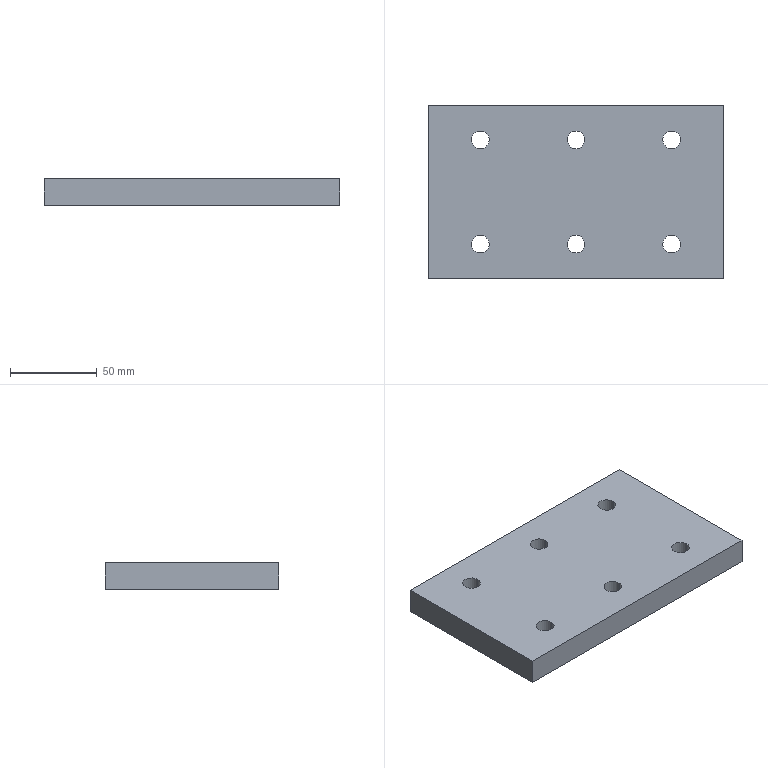Part | SolidWorks | features Extrusion 1, HoleWzd 1 | 1 solid | 18 faces | box 170 x 100 x 15 mm | volume 247646 mm3 | cylinder 12 | plane 6 | commonest cylinder face diameters 10.2 x12
STEP:
#1=CARTESIAN_POINT('',(-60.1,30.,0.));
#2=VERTEX_POINT('',#1);
#3=CARTESIAN_POINT('',(-49.9,30.,0.));
#4=VERTEX_POINT('',#3);
#5=CARTESIAN_POINT('',(-55.,30.,0.));
#6=DIRECTION('',(0.,0.,1.));
#7=DIRECTION('',(1.,0.,0.));
#8=AXIS2_PLACEMENT_3D('',#5,#6,#7);
#9=CIRCLE('',#8,5.1);
#10=EDGE_CURVE('',#2,#4,#9,.T.);
#11=ORIENTED_EDGE('',*,*,#10,.F.);
#12=CARTESIAN_POINT('',(-60.1,30.,15.));
#13=VERTEX_POINT('',#12);
#14=CARTESIAN_POINT('',(-60.1,30.,15.));
#15=DIRECTION('',(0.,0.,1.));
#16=VECTOR('',#15,1000.);
#17=LINE('',#14,#16);
#18=EDGE_CURVE('',#2,#13,#17,.T.);
#19=ORIENTED_EDGE('',*,*,#18,.T.);
#20=CARTESIAN_POINT('',(-49.9,30.,15.));
#21=VERTEX_POINT('',#20);
#22=CARTESIAN_POINT('',(-55.,30.,15.));
#23=DIRECTION('',(0.,0.,1.));
#24=DIRECTION('',(1.,0.,0.));
#25=AXIS2_PLACEMENT_3D('',#22,#23,#24);
#26=CIRCLE('',#25,5.1);
#27=EDGE_CURVE('',#13,#21,#26,.T.);
#28=ORIENTED_EDGE('',*,*,#27,.T.);
#29=CARTESIAN_POINT('',(-49.9,30.,15.));
#30=DIRECTION('',(0.,0.,1.));
#31=VECTOR('',#30,1000.);
#32=LINE('',#29,#31);
#33=EDGE_CURVE('',#4,#21,#32,.T.);
#34=ORIENTED_EDGE('',*,*,#33,.F.);
#35=EDGE_LOOP('',(#11,#19,#28,#34));
#36=FACE_OUTER_BOUND('',#35,.T.);
#37=CARTESIAN_POINT('',(-55.,30.,15.));
#38=DIRECTION('',(0.,0.,1.));
#39=DIRECTION('',(1.,0.,0.));
#40=AXIS2_PLACEMENT_3D('',#37,#38,#39);
#41=CYLINDRICAL_SURFACE('',#40,5.1);
#42=ADVANCED_FACE('',(#36),#41,.F.);
#43=CARTESIAN_POINT('',(-5.1,30.,0.));
#44=VERTEX_POINT('',#43);
#45=CARTESIAN_POINT('',(5.1,30.,0.));
#46=VERTEX_POINT('',#45);
#47=CARTESIAN_POINT('',(0.,30.,0.));
#48=DIRECTION('',(0.,0.,1.));
#49=DIRECTION('',(1.,0.,0.));
#50=AXIS2_PLACEMENT_3D('',#47,#48,#49);
#51=CIRCLE('',#50,5.1);
#52=EDGE_CURVE('',#44,#46,#51,.T.);
#53=ORIENTED_EDGE('',*,*,#52,.F.);
#54=CARTESIAN_POINT('',(-5.1,30.,15.));
#55=VERTEX_POINT('',#54);
#56=CARTESIAN_POINT('',(-5.1,30.,15.));
#57=DIRECTION('',(0.,0.,1.));
#58=VECTOR('',#57,1000.);
#59=LINE('',#56,#58);
#60=EDGE_CURVE('',#44,#55,#59,.T.);
#61=ORIENTED_EDGE('',*,*,#60,.T.);
#62=CARTESIAN_POINT('',(5.1,30.,15.));
#63=VERTEX_POINT('',#62);
#64=CARTESIAN_POINT('',(0.,30.,15.));
#65=DIRECTION('',(0.,0.,1.));
#66=DIRECTION('',(1.,0.,0.));
#67=AXIS2_PLACEMENT_3D('',#64,#65,#66);
#68=CIRCLE('',#67,5.1);
#69=EDGE_CURVE('',#55,#63,#68,.T.);
#70=ORIENTED_EDGE('',*,*,#69,.T.);
#71=CARTESIAN_POINT('',(5.1,30.,15.));
#72=DIRECTION('',(0.,0.,1.));
#73=VECTOR('',#72,1000.);
#74=LINE('',#71,#73);
#75=EDGE_CURVE('',#46,#63,#74,.T.);
#76=ORIENTED_EDGE('',*,*,#75,.F.);
#77=EDGE_LOOP('',(#53,#61,#70,#76));
#78=FACE_OUTER_BOUND('',#77,.T.);
#79=CARTESIAN_POINT('',(0.,30.,15.));
#80=DIRECTION('',(0.,0.,1.));
#81=DIRECTION('',(1.,0.,0.));
#82=AXIS2_PLACEMENT_3D('',#79,#80,#81);
#83=CYLINDRICAL_SURFACE('',#82,5.1);
#84=ADVANCED_FACE('',(#78),#83,.F.);
#85=CARTESIAN_POINT('',(49.9,30.,0.));
#86=VERTEX_POINT('',#85);
#87=CARTESIAN_POINT('',(60.1,30.,0.));
#88=VERTEX_POINT('',#87);
#89=CARTESIAN_POINT('',(55.,30.,0.));
#90=DIRECTION('',(0.,0.,1.));
#91=DIRECTION('',(1.,0.,0.));
#92=AXIS2_PLACEMENT_3D('',#89,#90,#91);
#93=CIRCLE('',#92,5.1);
#94=EDGE_CURVE('',#86,#88,#93,.T.);
#95=ORIENTED_EDGE('',*,*,#94,.F.);
#96=CARTESIAN_POINT('',(49.9,30.,15.));
#97=VERTEX_POINT('',#96);
#98=CARTESIAN_POINT('',(49.9,30.,15.));
#99=DIRECTION('',(0.,0.,1.));
#100=VECTOR('',#99,1000.);
#101=LINE('',#98,#100);
#102=EDGE_CURVE('',#86,#97,#101,.T.);
#103=ORIENTED_EDGE('',*,*,#102,.T.);
#104=CARTESIAN_POINT('',(60.1,30.,15.));
#105=VERTEX_POINT('',#104);
#106=CARTESIAN_POINT('',(55.,30.,15.));
#107=DIRECTION('',(0.,0.,1.));
#108=DIRECTION('',(1.,0.,0.));
#109=AXIS2_PLACEMENT_3D('',#106,#107,#108);
#110=CIRCLE('',#109,5.1);
#111=EDGE_CURVE('',#97,#105,#110,.T.);
#112=ORIENTED_EDGE('',*,*,#111,.T.);
#113=CARTESIAN_POINT('',(60.1,30.,15.));
#114=DIRECTION('',(0.,0.,1.));
#115=VECTOR('',#114,1000.);
#116=LINE('',#113,#115);
#117=EDGE_CURVE('',#88,#105,#116,.T.);
#118=ORIENTED_EDGE('',*,*,#117,.F.);
#119=EDGE_LOOP('',(#95,#103,#112,#118));
#120=FACE_OUTER_BOUND('',#119,.T.);
#121=CARTESIAN_POINT('',(55.,30.,15.));
#122=DIRECTION('',(0.,0.,1.));
#123=DIRECTION('',(1.,0.,0.));
#124=AXIS2_PLACEMENT_3D('',#121,#122,#123);
#125=CYLINDRICAL_SURFACE('',#124,5.1);
#126=ADVANCED_FACE('',(#120),#125,.F.);
#127=CARTESIAN_POINT('',(49.9,-30.,0.));
#128=VERTEX_POINT('',#127);
#129=CARTESIAN_POINT('',(60.1,-30.,0.));
#130=VERTEX_POINT('',#129);
#131=CARTESIAN_POINT('',(55.,-30.,0.));
#132=DIRECTION('',(0.,0.,1.));
#133=DIRECTION('',(1.,0.,0.));
#134=AXIS2_PLACEMENT_3D('',#131,#132,#133);
#135=CIRCLE('',#134,5.1);
#136=EDGE_CURVE('',#128,#130,#135,.T.);
#137=ORIENTED_EDGE('',*,*,#136,.F.);
#138=CARTESIAN_POINT('',(49.9,-30.,15.));
#139=VERTEX_POINT('',#138);
#140=CARTESIAN_POINT('',(49.9,-30.,15.));
#141=DIRECTION('',(0.,0.,1.));
#142=VECTOR('',#141,1000.);
#143=LINE('',#140,#142);
#144=EDGE_CURVE('',#128,#139,#143,.T.);
#145=ORIENTED_EDGE('',*,*,#144,.T.);
#146=CARTESIAN_POINT('',(60.1,-30.,15.));
#147=VERTEX_POINT('',#146);
#148=CARTESIAN_POINT('',(55.,-30.,15.));
#149=DIRECTION('',(0.,0.,1.));
#150=DIRECTION('',(1.,0.,0.));
#151=AXIS2_PLACEMENT_3D('',#148,#149,#150);
#152=CIRCLE('',#151,5.1);
#153=EDGE_CURVE('',#139,#147,#152,.T.);
#154=ORIENTED_EDGE('',*,*,#153,.T.);
#155=CARTESIAN_POINT('',(60.1,-30.,15.));
#156=DIRECTION('',(0.,0.,1.));
#157=VECTOR('',#156,1000.);
#158=LINE('',#155,#157);
#159=EDGE_CURVE('',#130,#147,#158,.T.);
#160=ORIENTED_EDGE('',*,*,#159,.F.);
#161=EDGE_LOOP('',(#137,#145,#154,#160));
#162=FACE_OUTER_BOUND('',#161,.T.);
#163=CARTESIAN_POINT('',(55.,-30.,15.));
#164=DIRECTION('',(0.,0.,1.));
#165=DIRECTION('',(1.,0.,0.));
#166=AXIS2_PLACEMENT_3D('',#163,#164,#165);
#167=CYLINDRICAL_SURFACE('',#166,5.1);
#168=ADVANCED_FACE('',(#162),#167,.F.);
#169=CARTESIAN_POINT('',(-5.1,-30.,0.));
#170=VERTEX_POINT('',#169);
#171=CARTESIAN_POINT('',(5.1,-30.,0.));
#172=VERTEX_POINT('',#171);
#173=CARTESIAN_POINT('',(0.,-30.,0.));
#174=DIRECTION('',(0.,0.,1.));
#175=DIRECTION('',(1.,0.,0.));
#176=AXIS2_PLACEMENT_3D('',#173,#174,#175);
#177=CIRCLE('',#176,5.1);
#178=EDGE_CURVE('',#170,#172,#177,.T.);
#179=ORIENTED_EDGE('',*,*,#178,.F.);
#180=CARTESIAN_POINT('',(-5.1,-30.,15.));
#181=VERTEX_POINT('',#180);
#182=CARTESIAN_POINT('',(-5.1,-30.,15.));
#183=DIRECTION('',(0.,0.,1.));
#184=VECTOR('',#183,1000.);
#185=LINE('',#182,#184);
#186=EDGE_CURVE('',#170,#181,#185,.T.);
#187=ORIENTED_EDGE('',*,*,#186,.T.);
#188=CARTESIAN_POINT('',(5.1,-30.,15.));
#189=VERTEX_POINT('',#188);
#190=CARTESIAN_POINT('',(0.,-30.,15.));
#191=DIRECTION('',(0.,0.,1.));
#192=DIRECTION('',(1.,0.,0.));
#193=AXIS2_PLACEMENT_3D('',#190,#191,#192);
#194=CIRCLE('',#193,5.1);
#195=EDGE_CURVE('',#181,#189,#194,.T.);
#196=ORIENTED_EDGE('',*,*,#195,.T.);
#197=CARTESIAN_POINT('',(5.1,-30.,15.));
#198=DIRECTION('',(0.,0.,1.));
#199=VECTOR('',#198,1000.);
#200=LINE('',#197,#199);
#201=EDGE_CURVE('',#172,#189,#200,.T.);
#202=ORIENTED_EDGE('',*,*,#201,.F.);
#203=EDGE_LOOP('',(#179,#187,#196,#202));
#204=FACE_OUTER_BOUND('',#203,.T.);
#205=CARTESIAN_POINT('',(0.,-30.,15.));
#206=DIRECTION('',(0.,0.,1.));
#207=DIRECTION('',(1.,0.,0.));
#208=AXIS2_PLACEMENT_3D('',#205,#206,#207);
#209=CYLINDRICAL_SURFACE('',#208,5.1);
#210=ADVANCED_FACE('',(#204),#209,.F.);
#211=CARTESIAN_POINT('',(-60.1,-30.,0.));
#212=VERTEX_POINT('',#211);
#213=CARTESIAN_POINT('',(-49.9,-30.,0.));
#214=VERTEX_POINT('',#213);
#215=CARTESIAN_POINT('',(-55.,-30.,0.));
#216=DIRECTION('',(0.,0.,1.));
#217=DIRECTION('',(1.,0.,0.));
#218=AXIS2_PLACEMENT_3D('',#215,#216,#217);
#219=CIRCLE('',#218,5.1);
#220=EDGE_CURVE('',#212,#214,#219,.T.);
#221=ORIENTED_EDGE('',*,*,#220,.F.);
#222=CARTESIAN_POINT('',(-60.1,-30.,15.));
#223=VERTEX_POINT('',#222);
#224=CARTESIAN_POINT('',(-60.1,-30.,15.));
#225=DIRECTION('',(0.,0.,1.));
#226=VECTOR('',#225,1000.);
#227=LINE('',#224,#226);
#228=EDGE_CURVE('',#212,#223,#227,.T.);
#229=ORIENTED_EDGE('',*,*,#228,.T.);
#230=CARTESIAN_POINT('',(-49.9,-30.,15.));
#231=VERTEX_POINT('',#230);
#232=CARTESIAN_POINT('',(-55.,-30.,15.));
#233=DIRECTION('',(0.,0.,1.));
#234=DIRECTION('',(1.,0.,0.));
#235=AXIS2_PLACEMENT_3D('',#232,#233,#234);
#236=CIRCLE('',#235,5.1);
#237=EDGE_CURVE('',#223,#231,#236,.T.);
#238=ORIENTED_EDGE('',*,*,#237,.T.);
#239=CARTESIAN_POINT('',(-49.9,-30.,15.));
#240=DIRECTION('',(0.,0.,1.));
#241=VECTOR('',#240,1000.);
#242=LINE('',#239,#241);
#243=EDGE_CURVE('',#214,#231,#242,.T.);
#244=ORIENTED_EDGE('',*,*,#243,.F.);
#245=EDGE_LOOP('',(#221,#229,#238,#244));
#246=FACE_OUTER_BOUND('',#245,.T.);
#247=CARTESIAN_POINT('',(-55.,-30.,15.));
#248=DIRECTION('',(0.,0.,1.));
#249=DIRECTION('',(1.,0.,0.));
#250=AXIS2_PLACEMENT_3D('',#247,#248,#249);
#251=CYLINDRICAL_SURFACE('',#250,5.1);
#252=ADVANCED_FACE('',(#246),#251,.F.);
#253=CARTESIAN_POINT('',(85.,-50.,0.));
#254=VERTEX_POINT('',#253);
#255=CARTESIAN_POINT('',(-85.,-50.,0.));
#256=VERTEX_POINT('',#255);
#257=CARTESIAN_POINT('',(85.,-50.,0.));
#258=DIRECTION('',(-1.,0.,0.));
#259=VECTOR('',#258,1000.);
#260=LINE('',#257,#259);
#261=EDGE_CURVE('',#254,#256,#260,.T.);
#262=ORIENTED_EDGE('',*,*,#261,.F.);
#263=CARTESIAN_POINT('',(85.,-50.,15.));
#264=VERTEX_POINT('',#263);
#265=CARTESIAN_POINT('',(85.,-50.,15.));
#266=DIRECTION('',(0.,0.,-1.));
#267=VECTOR('',#266,1000.);
#268=LINE('',#265,#267);
#269=EDGE_CURVE('',#264,#254,#268,.T.);
#270=ORIENTED_EDGE('',*,*,#269,.F.);
#271=CARTESIAN_POINT('',(-85.,-50.,15.));
#272=VERTEX_POINT('',#271);
#273=CARTESIAN_POINT('',(85.,-50.,15.));
#274=DIRECTION('',(-1.,0.,0.));
#275=VECTOR('',#274,1000.);
#276=LINE('',#273,#275);
#277=EDGE_CURVE('',#264,#272,#276,.T.);
#278=ORIENTED_EDGE('',*,*,#277,.T.);
#279=CARTESIAN_POINT('',(-85.,-50.,15.));
#280=DIRECTION('',(0.,0.,-1.));
#281=VECTOR('',#280,1000.);
#282=LINE('',#279,#281);
#283=EDGE_CURVE('',#272,#256,#282,.T.);
#284=ORIENTED_EDGE('',*,*,#283,.T.);
#285=EDGE_LOOP('',(#262,#270,#278,#284));
#286=FACE_OUTER_BOUND('',#285,.T.);
#287=CARTESIAN_POINT('',(85.,-50.,15.));
#288=DIRECTION('',(0.,-1.,0.));
#289=DIRECTION('',(1.,0.,0.));
#290=AXIS2_PLACEMENT_3D('',#287,#288,#289);
#291=PLANE('',#290);
#292=ADVANCED_FACE('',(#286),#291,.T.);
#293=CARTESIAN_POINT('',(85.,50.,0.));
#294=VERTEX_POINT('',#293);
#295=CARTESIAN_POINT('',(85.,50.,0.));
#296=DIRECTION('',(0.,-1.,0.));
#297=VECTOR('',#296,1000.);
#298=LINE('',#295,#297);
#299=EDGE_CURVE('',#294,#254,#298,.T.);
#300=ORIENTED_EDGE('',*,*,#299,.F.);
#301=CARTESIAN_POINT('',(85.,50.,15.));
#302=VERTEX_POINT('',#301);
#303=CARTESIAN_POINT('',(85.,50.,15.));
#304=DIRECTION('',(0.,0.,-1.));
#305=VECTOR('',#304,1000.);
#306=LINE('',#303,#305);
#307=EDGE_CURVE('',#302,#294,#306,.T.);
#308=ORIENTED_EDGE('',*,*,#307,.F.);
#309=CARTESIAN_POINT('',(85.,50.,15.));
#310=DIRECTION('',(0.,-1.,0.));
#311=VECTOR('',#310,1000.);
#312=LINE('',#309,#311);
#313=EDGE_CURVE('',#302,#264,#312,.T.);
#314=ORIENTED_EDGE('',*,*,#313,.T.);
#315=ORIENTED_EDGE('',*,*,#269,.T.);
#316=EDGE_LOOP('',(#300,#308,#314,#315));
#317=FACE_OUTER_BOUND('',#316,.T.);
#318=CARTESIAN_POINT('',(85.,50.,15.));
#319=DIRECTION('',(1.,0.,0.));
#320=DIRECTION('',(0.,1.,0.));
#321=AXIS2_PLACEMENT_3D('',#318,#319,#320);
#322=PLANE('',#321);
#323=ADVANCED_FACE('',(#317),#322,.T.);
#324=CARTESIAN_POINT('',(-85.,50.,0.));
#325=VERTEX_POINT('',#324);
#326=CARTESIAN_POINT('',(85.,50.,0.));
#327=DIRECTION('',(-1.,0.,0.));
#328=VECTOR('',#327,1000.);
#329=LINE('',#326,#328);
#330=EDGE_CURVE('',#294,#325,#329,.T.);
#331=ORIENTED_EDGE('',*,*,#330,.T.);
#332=CARTESIAN_POINT('',(-85.,50.,15.));
#333=VERTEX_POINT('',#332);
#334=CARTESIAN_POINT('',(-85.,50.,15.));
#335=DIRECTION('',(0.,0.,-1.));
#336=VECTOR('',#335,1000.);
#337=LINE('',#334,#336);
#338=EDGE_CURVE('',#333,#325,#337,.T.);
#339=ORIENTED_EDGE('',*,*,#338,.F.);
#340=CARTESIAN_POINT('',(85.,50.,15.));
#341=DIRECTION('',(-1.,0.,0.));
#342=VECTOR('',#341,1000.);
#343=LINE('',#340,#342);
#344=EDGE_CURVE('',#302,#333,#343,.T.);
#345=ORIENTED_EDGE('',*,*,#344,.F.);
#346=ORIENTED_EDGE('',*,*,#307,.T.);
#347=EDGE_LOOP('',(#331,#339,#345,#346));
#348=FACE_OUTER_BOUND('',#347,.T.);
#349=CARTESIAN_POINT('',(85.,50.,15.));
#350=DIRECTION('',(0.,-1.,0.));
#351=DIRECTION('',(1.,0.,0.));
#352=AXIS2_PLACEMENT_3D('',#349,#350,#351);
#353=PLANE('',#352);
#354=ADVANCED_FACE('',(#348),#353,.F.);
#355=CARTESIAN_POINT('',(-85.,50.,0.));
#356=DIRECTION('',(0.,-1.,0.));
#357=VECTOR('',#356,1000.);
#358=LINE('',#355,#357);
#359=EDGE_CURVE('',#325,#256,#358,.T.);
#360=ORIENTED_EDGE('',*,*,#359,.T.);
#361=ORIENTED_EDGE('',*,*,#283,.F.);
#362=CARTESIAN_POINT('',(-85.,50.,15.));
#363=DIRECTION('',(0.,-1.,0.));
#364=VECTOR('',#363,1000.);
#365=LINE('',#362,#364);
#366=EDGE_CURVE('',#333,#272,#365,.T.);
#367=ORIENTED_EDGE('',*,*,#366,.F.);
#368=ORIENTED_EDGE('',*,*,#338,.T.);
#369=EDGE_LOOP('',(#360,#361,#367,#368));
#370=FACE_OUTER_BOUND('',#369,.T.);
#371=CARTESIAN_POINT('',(-85.,50.,15.));
#372=DIRECTION('',(1.,0.,0.));
#373=DIRECTION('',(0.,1.,0.));
#374=AXIS2_PLACEMENT_3D('',#371,#372,#373);
#375=PLANE('',#374);
#376=ADVANCED_FACE('',(#370),#375,.F.);
#377=CARTESIAN_POINT('',(-55.,30.,15.));
#378=DIRECTION('',(0.,0.,1.));
#379=DIRECTION('',(1.,0.,0.));
#380=AXIS2_PLACEMENT_3D('',#377,#378,#379);
#381=CIRCLE('',#380,5.1);
#382=EDGE_CURVE('',#21,#13,#381,.T.);
#383=ORIENTED_EDGE('',*,*,#382,.F.);
#384=ORIENTED_EDGE('',*,*,#27,.F.);
#385=EDGE_LOOP('',(#383,#384));
#386=FACE_BOUND('',#385,.T.);
#387=CARTESIAN_POINT('',(0.,30.,15.));
#388=DIRECTION('',(0.,0.,1.));
#389=DIRECTION('',(1.,0.,0.));
#390=AXIS2_PLACEMENT_3D('',#387,#388,#389);
#391=CIRCLE('',#390,5.1);
#392=EDGE_CURVE('',#63,#55,#391,.T.);
#393=ORIENTED_EDGE('',*,*,#392,.F.);
#394=ORIENTED_EDGE('',*,*,#69,.F.);
#395=EDGE_LOOP('',(#393,#394));
#396=FACE_BOUND('',#395,.T.);
#397=CARTESIAN_POINT('',(55.,30.,15.));
#398=DIRECTION('',(0.,0.,1.));
#399=DIRECTION('',(1.,0.,0.));
#400=AXIS2_PLACEMENT_3D('',#397,#398,#399);
#401=CIRCLE('',#400,5.1);
#402=EDGE_CURVE('',#105,#97,#401,.T.);
#403=ORIENTED_EDGE('',*,*,#402,.F.);
#404=ORIENTED_EDGE('',*,*,#111,.F.);
#405=EDGE_LOOP('',(#403,#404));
#406=FACE_BOUND('',#405,.T.);
#407=CARTESIAN_POINT('',(55.,-30.,15.));
#408=DIRECTION('',(0.,0.,1.));
#409=DIRECTION('',(1.,0.,0.));
#410=AXIS2_PLACEMENT_3D('',#407,#408,#409);
#411=CIRCLE('',#410,5.1);
#412=EDGE_CURVE('',#147,#139,#411,.T.);
#413=ORIENTED_EDGE('',*,*,#412,.F.);
#414=ORIENTED_EDGE('',*,*,#153,.F.);
#415=EDGE_LOOP('',(#413,#414));
#416=FACE_BOUND('',#415,.T.);
#417=CARTESIAN_POINT('',(0.,-30.,15.));
#418=DIRECTION('',(0.,0.,1.));
#419=DIRECTION('',(1.,0.,0.));
#420=AXIS2_PLACEMENT_3D('',#417,#418,#419);
#421=CIRCLE('',#420,5.1);
#422=EDGE_CURVE('',#189,#181,#421,.T.);
#423=ORIENTED_EDGE('',*,*,#422,.F.);
#424=ORIENTED_EDGE('',*,*,#195,.F.);
#425=EDGE_LOOP('',(#423,#424));
#426=FACE_BOUND('',#425,.T.);
#427=CARTESIAN_POINT('',(-55.,-30.,15.));
#428=DIRECTION('',(0.,0.,1.));
#429=DIRECTION('',(1.,0.,0.));
#430=AXIS2_PLACEMENT_3D('',#427,#428,#429);
#431=CIRCLE('',#430,5.1);
#432=EDGE_CURVE('',#231,#223,#431,.T.);
#433=ORIENTED_EDGE('',*,*,#432,.F.);
#434=ORIENTED_EDGE('',*,*,#237,.F.);
#435=EDGE_LOOP('',(#433,#434));
#436=FACE_BOUND('',#435,.T.);
#437=ORIENTED_EDGE('',*,*,#277,.F.);
#438=ORIENTED_EDGE('',*,*,#313,.F.);
#439=ORIENTED_EDGE('',*,*,#344,.T.);
#440=ORIENTED_EDGE('',*,*,#366,.T.);
#441=EDGE_LOOP('',(#437,#438,#439,#440));
#442=FACE_OUTER_BOUND('',#441,.T.);
#443=CARTESIAN_POINT('',(0.,0.,15.));
#444=DIRECTION('',(0.,0.,1.));
#445=DIRECTION('',(1.,0.,0.));
#446=AXIS2_PLACEMENT_3D('',#443,#444,#445);
#447=PLANE('',#446);
#448=ADVANCED_FACE('',(#386,#396,#406,#416,#426,#436,#442),#447,.T.);
#449=CARTESIAN_POINT('',(-55.,30.,0.));
#450=DIRECTION('',(0.,0.,1.));
#451=DIRECTION('',(1.,0.,0.));
#452=AXIS2_PLACEMENT_3D('',#449,#450,#451);
#453=CIRCLE('',#452,5.1);
#454=EDGE_CURVE('',#4,#2,#453,.T.);
#455=ORIENTED_EDGE('',*,*,#454,.T.);
#456=ORIENTED_EDGE('',*,*,#10,.T.);
#457=EDGE_LOOP('',(#455,#456));
#458=FACE_BOUND('',#457,.T.);
#459=CARTESIAN_POINT('',(0.,30.,0.));
#460=DIRECTION('',(0.,0.,1.));
#461=DIRECTION('',(1.,0.,0.));
#462=AXIS2_PLACEMENT_3D('',#459,#460,#461);
#463=CIRCLE('',#462,5.1);
#464=EDGE_CURVE('',#46,#44,#463,.T.);
#465=ORIENTED_EDGE('',*,*,#464,.T.);
#466=ORIENTED_EDGE('',*,*,#52,.T.);
#467=EDGE_LOOP('',(#465,#466));
#468=FACE_BOUND('',#467,.T.);
#469=CARTESIAN_POINT('',(55.,30.,0.));
#470=DIRECTION('',(0.,0.,1.));
#471=DIRECTION('',(1.,0.,0.));
#472=AXIS2_PLACEMENT_3D('',#469,#470,#471);
#473=CIRCLE('',#472,5.1);
#474=EDGE_CURVE('',#88,#86,#473,.T.);
#475=ORIENTED_EDGE('',*,*,#474,.T.);
#476=ORIENTED_EDGE('',*,*,#94,.T.);
#477=EDGE_LOOP('',(#475,#476));
#478=FACE_BOUND('',#477,.T.);
#479=CARTESIAN_POINT('',(55.,-30.,0.));
#480=DIRECTION('',(0.,0.,1.));
#481=DIRECTION('',(1.,0.,0.));
#482=AXIS2_PLACEMENT_3D('',#479,#480,#481);
#483=CIRCLE('',#482,5.1);
#484=EDGE_CURVE('',#130,#128,#483,.T.);
#485=ORIENTED_EDGE('',*,*,#484,.T.);
#486=ORIENTED_EDGE('',*,*,#136,.T.);
#487=EDGE_LOOP('',(#485,#486));
#488=FACE_BOUND('',#487,.T.);
#489=CARTESIAN_POINT('',(0.,-30.,0.));
#490=DIRECTION('',(0.,0.,1.));
#491=DIRECTION('',(1.,0.,0.));
#492=AXIS2_PLACEMENT_3D('',#489,#490,#491);
#493=CIRCLE('',#492,5.1);
#494=EDGE_CURVE('',#172,#170,#493,.T.);
#495=ORIENTED_EDGE('',*,*,#494,.T.);
#496=ORIENTED_EDGE('',*,*,#178,.T.);
#497=EDGE_LOOP('',(#495,#496));
#498=FACE_BOUND('',#497,.T.);
#499=CARTESIAN_POINT('',(-55.,-30.,0.));
#500=DIRECTION('',(0.,0.,1.));
#501=DIRECTION('',(1.,0.,0.));
#502=AXIS2_PLACEMENT_3D('',#499,#500,#501);
#503=CIRCLE('',#502,5.1);
#504=EDGE_CURVE('',#214,#212,#503,.T.);
#505=ORIENTED_EDGE('',*,*,#504,.T.);
#506=ORIENTED_EDGE('',*,*,#220,.T.);
#507=EDGE_LOOP('',(#505,#506));
#508=FACE_BOUND('',#507,.T.);
#509=ORIENTED_EDGE('',*,*,#261,.T.);
#510=ORIENTED_EDGE('',*,*,#359,.F.);
#511=ORIENTED_EDGE('',*,*,#330,.F.);
#512=ORIENTED_EDGE('',*,*,#299,.T.);
#513=EDGE_LOOP('',(#509,#510,#511,#512));
#514=FACE_OUTER_BOUND('',#513,.T.);
#515=CARTESIAN_POINT('',(0.,0.,0.));
#516=DIRECTION('',(0.,0.,1.));
#517=DIRECTION('',(1.,0.,0.));
#518=AXIS2_PLACEMENT_3D('',#515,#516,#517);
#519=PLANE('',#518);
#520=ADVANCED_FACE('',(#458,#468,#478,#488,#498,#508,#514),#519,.F.);
#521=ORIENTED_EDGE('',*,*,#228,.F.);
#522=ORIENTED_EDGE('',*,*,#504,.F.);
#523=ORIENTED_EDGE('',*,*,#243,.T.);
#524=ORIENTED_EDGE('',*,*,#432,.T.);
#525=EDGE_LOOP('',(#521,#522,#523,#524));
#526=FACE_OUTER_BOUND('',#525,.T.);
#527=CARTESIAN_POINT('',(-55.,-30.,15.));
#528=DIRECTION('',(0.,0.,1.));
#529=DIRECTION('',(1.,0.,0.));
#530=AXIS2_PLACEMENT_3D('',#527,#528,#529);
#531=CYLINDRICAL_SURFACE('',#530,5.1);
#532=ADVANCED_FACE('',(#526),#531,.F.);
#533=ORIENTED_EDGE('',*,*,#186,.F.);
#534=ORIENTED_EDGE('',*,*,#494,.F.);
#535=ORIENTED_EDGE('',*,*,#201,.T.);
#536=ORIENTED_EDGE('',*,*,#422,.T.);
#537=EDGE_LOOP('',(#533,#534,#535,#536));
#538=FACE_OUTER_BOUND('',#537,.T.);
#539=CARTESIAN_POINT('',(0.,-30.,15.));
#540=DIRECTION('',(0.,0.,1.));
#541=DIRECTION('',(1.,0.,0.));
#542=AXIS2_PLACEMENT_3D('',#539,#540,#541);
#543=CYLINDRICAL_SURFACE('',#542,5.1);
#544=ADVANCED_FACE('',(#538),#543,.F.);
#545=ORIENTED_EDGE('',*,*,#144,.F.);
#546=ORIENTED_EDGE('',*,*,#484,.F.);
#547=ORIENTED_EDGE('',*,*,#159,.T.);
#548=ORIENTED_EDGE('',*,*,#412,.T.);
#549=EDGE_LOOP('',(#545,#546,#547,#548));
#550=FACE_OUTER_BOUND('',#549,.T.);
#551=CARTESIAN_POINT('',(55.,-30.,15.));
#552=DIRECTION('',(0.,0.,1.));
#553=DIRECTION('',(1.,0.,0.));
#554=AXIS2_PLACEMENT_3D('',#551,#552,#553);
#555=CYLINDRICAL_SURFACE('',#554,5.1);
#556=ADVANCED_FACE('',(#550),#555,.F.);
#557=ORIENTED_EDGE('',*,*,#102,.F.);
#558=ORIENTED_EDGE('',*,*,#474,.F.);
#559=ORIENTED_EDGE('',*,*,#117,.T.);
#560=ORIENTED_EDGE('',*,*,#402,.T.);
#561=EDGE_LOOP('',(#557,#558,#559,#560));
#562=FACE_OUTER_BOUND('',#561,.T.);
#563=CARTESIAN_POINT('',(55.,30.,15.));
#564=DIRECTION('',(0.,0.,1.));
#565=DIRECTION('',(1.,0.,0.));
#566=AXIS2_PLACEMENT_3D('',#563,#564,#565);
#567=CYLINDRICAL_SURFACE('',#566,5.1);
#568=ADVANCED_FACE('',(#562),#567,.F.);
#569=ORIENTED_EDGE('',*,*,#60,.F.);
#570=ORIENTED_EDGE('',*,*,#464,.F.);
#571=ORIENTED_EDGE('',*,*,#75,.T.);
#572=ORIENTED_EDGE('',*,*,#392,.T.);
#573=EDGE_LOOP('',(#569,#570,#571,#572));
#574=FACE_OUTER_BOUND('',#573,.T.);
#575=CARTESIAN_POINT('',(0.,30.,15.));
#576=DIRECTION('',(0.,0.,1.));
#577=DIRECTION('',(1.,0.,0.));
#578=AXIS2_PLACEMENT_3D('',#575,#576,#577);
#579=CYLINDRICAL_SURFACE('',#578,5.1);
#580=ADVANCED_FACE('',(#574),#579,.F.);
#581=ORIENTED_EDGE('',*,*,#18,.F.);
#582=ORIENTED_EDGE('',*,*,#454,.F.);
#583=ORIENTED_EDGE('',*,*,#33,.T.);
#584=ORIENTED_EDGE('',*,*,#382,.T.);
#585=EDGE_LOOP('',(#581,#582,#583,#584));
#586=FACE_OUTER_BOUND('',#585,.T.);
#587=CARTESIAN_POINT('',(-55.,30.,15.));
#588=DIRECTION('',(0.,0.,1.));
#589=DIRECTION('',(1.,0.,0.));
#590=AXIS2_PLACEMENT_3D('',#587,#588,#589);
#591=CYLINDRICAL_SURFACE('',#590,5.1);
#592=ADVANCED_FACE('',(#586),#591,.F.);
#593=CLOSED_SHELL('',(#42,#84,#126,#168,#210,#252,#292,#323,#354,#376,#448,#520,#532,#544,#556,#568,#580,#592));
#594=MANIFOLD_SOLID_BREP('',#593);
#595=CARTESIAN_POINT('',(0.,0.,0.));
#596=DIRECTION('',(0.,0.,1.));
#597=DIRECTION('',(1.,0.,0.));
#598=AXIS2_PLACEMENT_3D('',#595,#596,#597);
#599=(LENGTH_UNIT()NAMED_UNIT(*)SI_UNIT(.MILLI.,.METRE.));
#600=UNCERTAINTY_MEASURE_WITH_UNIT(LENGTH_MEASURE(0.00001),#599,'','');
#601=(NAMED_UNIT(*)PLANE_ANGLE_UNIT()SI_UNIT($,.RADIAN.));
#602=(NAMED_UNIT(*)SI_UNIT($,.STERADIAN.)SOLID_ANGLE_UNIT());
#603=(GEOMETRIC_REPRESENTATION_CONTEXT(3)GLOBAL_UNCERTAINTY_ASSIGNED_CONTEXT((#600))GLOBAL_UNIT_ASSIGNED_CONTEXT((#599,#601,#602))REPRESENTATION_CONTEXT('',''));
#604=ADVANCED_BREP_SHAPE_REPRESENTATION('',(#594,#598),#603);